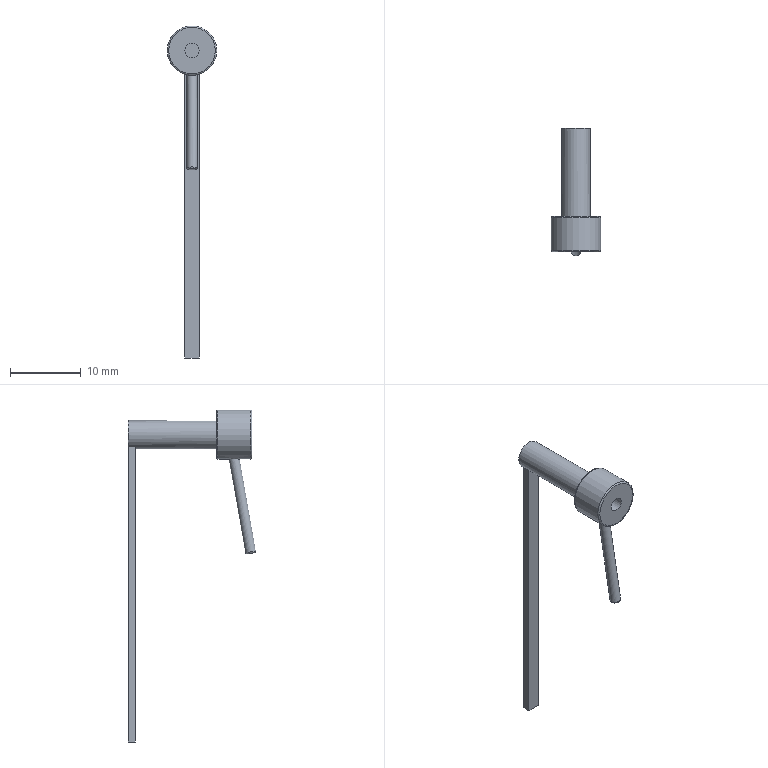Part | STEP file | 1-35.1 | 1 solid | 16 faces | box 7 x 18.051 x 47 mm | volume 449.87 mm3 | plane 9 | cylinder 4 | torus 3 | commonest cylinder face diameters 1.5 x1 2 x1 4 x1 7 x1
STEP:
#1=CARTESIAN_POINT('',(0.,0.,0.));
#2=DIRECTION('',(0.,0.,1.));
#3=DIRECTION('',(1.,0.,0.));
#4=AXIS2_PLACEMENT_3D('',#1,#2,#3);
#5=CARTESIAN_POINT('',(-1.,11.5,-1.732));
#6=VERTEX_POINT('',#5);
#7=CARTESIAN_POINT('',(1.,11.5,-1.732));
#8=VERTEX_POINT('',#7);
#9=CARTESIAN_POINT('',(0.,11.5,0.));
#10=DIRECTION('',(0.,-1.,0.));
#11=DIRECTION('',(-0.5,0.,-0.866));
#12=AXIS2_PLACEMENT_3D('',#9,#10,#11);
#13=CIRCLE('',#12,2.);
#14=CARTESIAN_POINT('',(0.,0.,0.));
#15=DIRECTION('',(0.,1.,0.));
#16=DIRECTION('',(1.,0.,0.));
#17=AXIS2_PLACEMENT_3D('',#14,#15,#16);
#18=CYLINDRICAL_SURFACE('',#17,2.);
#19=CARTESIAN_POINT('',(2.094,11.5));
#20=DIRECTION('',(-1.,0.));
#21=VECTOR('',#20,1.);
#22=LINE('',#19,#21);
#23=(GEOMETRIC_REPRESENTATION_CONTEXT(2)PARAMETRIC_REPRESENTATION_CONTEXT()REPRESENTATION_CONTEXT('',''));
#24=DEFINITIONAL_REPRESENTATION('',(#22),#23);
#25=PCURVE('',#18,#24);
#26=CARTESIAN_POINT('',(-20.242,11.5,-20.194));
#27=DIRECTION('',(0.,1.,0.));
#28=DIRECTION('',(-1.,0.,0.));
#29=AXIS2_PLACEMENT_3D('',#26,#27,#28);
#30=PLANE('',#29);
#31=CARTESIAN_POINT('',(-19.242,18.462));
#32=CARTESIAN_POINT('',(-22.242,16.73));
#33=CARTESIAN_POINT('',(-22.242,20.194));
#34=CARTESIAN_POINT('',(-22.242,23.658));
#35=CARTESIAN_POINT('',(-19.242,21.926));
#36=CARTESIAN_POINT('',(-16.242,20.194));
#37=CARTESIAN_POINT('',(-19.242,18.462));
#38=(BOUNDED_CURVE()B_SPLINE_CURVE(2,(#31,#32,#33,#34,#35,#36,#37),.UNSPECIFIED.,.T.,.F.)B_SPLINE_CURVE_WITH_KNOTS((1,2,2,2,2,1),(-2.094,0.,2.094,4.189,6.283,8.378),.UNSPECIFIED.)CURVE()GEOMETRIC_REPRESENTATION_ITEM()RATIONAL_B_SPLINE_CURVE((1.,0.5,1.,0.5,1.,0.5,1.))REPRESENTATION_ITEM(''));
#39=(GEOMETRIC_REPRESENTATION_CONTEXT(2)PARAMETRIC_REPRESENTATION_CONTEXT()REPRESENTATION_CONTEXT('',''));
#40=DEFINITIONAL_REPRESENTATION('',(#38),#39);
#41=PCURVE('',#30,#40);
#42=SURFACE_CURVE('',#13,(#25,#41),.PCURVE_S1.);
#43=EDGE_CURVE('',#6,#8,#42,.T.);
#44=ORIENTED_EDGE('',*,*,#43,.T.);
#45=CARTESIAN_POINT('',(1.,12.5,-1.732));
#46=VERTEX_POINT('',#45);
#47=CARTESIAN_POINT('',(1.,11.5,-1.732));
#48=DIRECTION('',(0.,1.,0.));
#49=VECTOR('',#48,1.);
#50=LINE('',#47,#49);
#51=CARTESIAN_POINT('',(1.047,11.5));
#52=DIRECTION('',(0.,1.));
#53=VECTOR('',#52,1.);
#54=LINE('',#51,#53);
#55=(GEOMETRIC_REPRESENTATION_CONTEXT(2)PARAMETRIC_REPRESENTATION_CONTEXT()REPRESENTATION_CONTEXT('',''));
#56=DEFINITIONAL_REPRESENTATION('',(#54),#55);
#57=PCURVE('',#18,#56);
#58=CARTESIAN_POINT('',(1.,12.,-22.616));
#59=DIRECTION('',(1.,0.,0.));
#60=DIRECTION('',(0.,0.,-1.));
#61=AXIS2_PLACEMENT_3D('',#58,#59,#60);
#62=PLANE('',#61);
#63=CARTESIAN_POINT('',(-20.884,-0.5));
#64=DIRECTION('',(0.,1.));
#65=VECTOR('',#64,1.);
#66=LINE('',#63,#65);
#67=(GEOMETRIC_REPRESENTATION_CONTEXT(2)PARAMETRIC_REPRESENTATION_CONTEXT()REPRESENTATION_CONTEXT('',''));
#68=DEFINITIONAL_REPRESENTATION('',(#66),#67);
#69=PCURVE('',#62,#68);
#70=SURFACE_CURVE('',#50,(#57,#69),.PCURVE_S1.);
#71=EDGE_CURVE('',#8,#46,#70,.T.);
#72=ORIENTED_EDGE('',*,*,#71,.T.);
#73=CARTESIAN_POINT('',(2.,12.5,0.));
#74=VERTEX_POINT('',#73);
#75=CARTESIAN_POINT('',(0.,12.5,0.));
#76=DIRECTION('',(0.,1.,0.));
#77=DIRECTION('',(1.,0.,0.));
#78=AXIS2_PLACEMENT_3D('',#75,#76,#77);
#79=CIRCLE('',#78,2.);
#80=CARTESIAN_POINT('',(0.,12.5));
#81=DIRECTION('',(1.,0.));
#82=VECTOR('',#81,1.);
#83=LINE('',#80,#82);
#84=(GEOMETRIC_REPRESENTATION_CONTEXT(2)PARAMETRIC_REPRESENTATION_CONTEXT()REPRESENTATION_CONTEXT('',''));
#85=DEFINITIONAL_REPRESENTATION('',(#83),#84);
#86=PCURVE('',#18,#85);
#87=CARTESIAN_POINT('',(-20.242,12.5,-20.194));
#88=DIRECTION('',(0.,1.,0.));
#89=DIRECTION('',(-1.,0.,0.));
#90=AXIS2_PLACEMENT_3D('',#87,#88,#89);
#91=PLANE('',#90);
#92=CARTESIAN_POINT('',(-20.242,20.194));
#93=DIRECTION('',(-1.,0.));
#94=AXIS2_PLACEMENT_2D('',#92,#93);
#95=CIRCLE('',#94,2.);
#96=(GEOMETRIC_REPRESENTATION_CONTEXT(2)PARAMETRIC_REPRESENTATION_CONTEXT()REPRESENTATION_CONTEXT('',''));
#97=DEFINITIONAL_REPRESENTATION('',(#95),#96);
#98=PCURVE('',#91,#97);
#99=SURFACE_CURVE('',#79,(#86,#98),.PCURVE_S1.);
#100=EDGE_CURVE('',#74,#46,#99,.T.);
#101=ORIENTED_EDGE('',*,*,#100,.F.);
#102=CARTESIAN_POINT('',(2.,0.,0.));
#103=VERTEX_POINT('',#102);
#104=CARTESIAN_POINT('',(2.,0.,0.));
#105=DIRECTION('',(0.,1.,0.));
#106=VECTOR('',#105,1.);
#107=LINE('',#104,#106);
#108=CARTESIAN_POINT('',(0.,0.));
#109=DIRECTION('',(0.,1.));
#110=VECTOR('',#109,1.);
#111=LINE('',#108,#110);
#112=(GEOMETRIC_REPRESENTATION_CONTEXT(2)PARAMETRIC_REPRESENTATION_CONTEXT()REPRESENTATION_CONTEXT('',''));
#113=DEFINITIONAL_REPRESENTATION('',(#111),#112);
#114=PCURVE('',#18,#113);
#115=CARTESIAN_POINT('',(6.283,0.));
#116=DIRECTION('',(0.,1.));
#117=VECTOR('',#116,1.);
#118=LINE('',#115,#117);
#119=(GEOMETRIC_REPRESENTATION_CONTEXT(2)PARAMETRIC_REPRESENTATION_CONTEXT()REPRESENTATION_CONTEXT('',''));
#120=DEFINITIONAL_REPRESENTATION('',(#118),#119);
#121=PCURVE('',#18,#120);
#122=SEAM_CURVE('',#107,(#114,#121),.PCURVE_S1.);
#123=EDGE_CURVE('',#103,#74,#122,.T.);
#124=ORIENTED_EDGE('',*,*,#123,.F.);
#125=CARTESIAN_POINT('',(0.,0.,0.));
#126=DIRECTION('',(0.,-1.,0.));
#127=DIRECTION('',(1.,0.,0.));
#128=AXIS2_PLACEMENT_3D('',#125,#126,#127);
#129=CIRCLE('',#128,2.);
#130=CARTESIAN_POINT('',(6.283,0.));
#131=DIRECTION('',(-1.,0.));
#132=VECTOR('',#131,1.);
#133=LINE('',#130,#132);
#134=(GEOMETRIC_REPRESENTATION_CONTEXT(2)PARAMETRIC_REPRESENTATION_CONTEXT()REPRESENTATION_CONTEXT('',''));
#135=DEFINITIONAL_REPRESENTATION('',(#133),#134);
#136=PCURVE('',#18,#135);
#137=CARTESIAN_POINT('',(-0.9378,0.,0.));
#138=DIRECTION('',(0.,-1.,0.));
#139=DIRECTION('',(1.,0.,0.));
#140=AXIS2_PLACEMENT_3D('',#137,#138,#139);
#141=PLANE('',#140);
#142=CARTESIAN_POINT('',(0.9378,0.));
#143=DIRECTION('',(1.,0.));
#144=AXIS2_PLACEMENT_2D('',#142,#143);
#145=CIRCLE('',#144,2.);
#146=(GEOMETRIC_REPRESENTATION_CONTEXT(2)PARAMETRIC_REPRESENTATION_CONTEXT()REPRESENTATION_CONTEXT('',''));
#147=DEFINITIONAL_REPRESENTATION('',(#145),#146);
#148=PCURVE('',#141,#147);
#149=SURFACE_CURVE('',#129,(#136,#148),.PCURVE_S1.);
#150=EDGE_CURVE('',#103,#103,#149,.T.);
#151=ORIENTED_EDGE('',*,*,#150,.F.);
#152=ORIENTED_EDGE('',*,*,#123,.T.);
#153=CARTESIAN_POINT('',(-1.,12.5,-1.732));
#154=VERTEX_POINT('',#153);
#155=CARTESIAN_POINT('',(0.,12.5,0.));
#156=DIRECTION('',(0.,1.,0.));
#157=DIRECTION('',(-0.5,0.,-0.866));
#158=AXIS2_PLACEMENT_3D('',#155,#156,#157);
#159=CIRCLE('',#158,2.);
#160=CARTESIAN_POINT('',(2.094,12.5));
#161=DIRECTION('',(1.,0.));
#162=VECTOR('',#161,1.);
#163=LINE('',#160,#162);
#164=(GEOMETRIC_REPRESENTATION_CONTEXT(2)PARAMETRIC_REPRESENTATION_CONTEXT()REPRESENTATION_CONTEXT('',''));
#165=DEFINITIONAL_REPRESENTATION('',(#163),#164);
#166=PCURVE('',#18,#165);
#167=CARTESIAN_POINT('',(-20.242,20.194));
#168=DIRECTION('',(0.5,-0.866));
#169=AXIS2_PLACEMENT_2D('',#167,#168);
#170=CIRCLE('',#169,2.);
#171=(GEOMETRIC_REPRESENTATION_CONTEXT(2)PARAMETRIC_REPRESENTATION_CONTEXT()REPRESENTATION_CONTEXT('',''));
#172=DEFINITIONAL_REPRESENTATION('',(#170),#171);
#173=PCURVE('',#91,#172);
#174=SURFACE_CURVE('',#159,(#166,#173),.PCURVE_S1.);
#175=EDGE_CURVE('',#154,#74,#174,.T.);
#176=ORIENTED_EDGE('',*,*,#175,.F.);
#177=CARTESIAN_POINT('',(-1.,11.5,-1.732));
#178=DIRECTION('',(0.,1.,0.));
#179=VECTOR('',#178,1.);
#180=LINE('',#177,#179);
#181=CARTESIAN_POINT('',(2.094,11.5));
#182=DIRECTION('',(0.,1.));
#183=VECTOR('',#182,1.);
#184=LINE('',#181,#183);
#185=(GEOMETRIC_REPRESENTATION_CONTEXT(2)PARAMETRIC_REPRESENTATION_CONTEXT()REPRESENTATION_CONTEXT('',''));
#186=DEFINITIONAL_REPRESENTATION('',(#184),#185);
#187=PCURVE('',#18,#186);
#188=CARTESIAN_POINT('',(-1.,12.,-22.616));
#189=DIRECTION('',(-1.,0.,0.));
#190=DIRECTION('',(0.,0.,1.));
#191=AXIS2_PLACEMENT_3D('',#188,#189,#190);
#192=PLANE('',#191);
#193=CARTESIAN_POINT('',(20.884,-0.5));
#194=DIRECTION('',(0.,1.));
#195=VECTOR('',#194,1.);
#196=LINE('',#193,#195);
#197=(GEOMETRIC_REPRESENTATION_CONTEXT(2)PARAMETRIC_REPRESENTATION_CONTEXT()REPRESENTATION_CONTEXT('',''));
#198=DEFINITIONAL_REPRESENTATION('',(#196),#197);
#199=PCURVE('',#192,#198);
#200=SURFACE_CURVE('',#180,(#187,#199),.PCURVE_S1.);
#201=EDGE_CURVE('',#6,#154,#200,.T.);
#202=ORIENTED_EDGE('',*,*,#201,.F.);
#203=EDGE_LOOP('',(#44,#72,#101,#124,#151,#152,#176,#202));
#204=FACE_BOUND('',#203,.T.);
#205=ADVANCED_FACE('',(#204),#18,.T.);
#206=CARTESIAN_POINT('',(3.3,0.,0.));
#207=VERTEX_POINT('',#206);
#208=CARTESIAN_POINT('',(0.,0.,0.));
#209=DIRECTION('',(0.,1.,0.));
#210=DIRECTION('',(1.,0.,0.));
#211=AXIS2_PLACEMENT_3D('',#208,#209,#210);
#212=CIRCLE('',#211,3.3);
#213=CARTESIAN_POINT('',(4.238,0.));
#214=CARTESIAN_POINT('',(4.238,-5.716));
#215=CARTESIAN_POINT('',(-0.7122,-2.858));
#216=CARTESIAN_POINT('',(-5.662,0.));
#217=CARTESIAN_POINT('',(-0.7122,2.858));
#218=CARTESIAN_POINT('',(4.238,5.716));
#219=CARTESIAN_POINT('',(4.238,0.));
#220=(BOUNDED_CURVE()B_SPLINE_CURVE(2,(#213,#214,#215,#216,#217,#218,#219),.UNSPECIFIED.,.T.,.F.)B_SPLINE_CURVE_WITH_KNOTS((1,2,2,2,2,1),(-2.094,0.,2.094,4.189,6.283,8.378),.UNSPECIFIED.)CURVE()GEOMETRIC_REPRESENTATION_ITEM()RATIONAL_B_SPLINE_CURVE((1.,0.5,1.,0.5,1.,0.5,1.))REPRESENTATION_ITEM(''));
#221=(GEOMETRIC_REPRESENTATION_CONTEXT(2)PARAMETRIC_REPRESENTATION_CONTEXT()REPRESENTATION_CONTEXT('',''));
#222=DEFINITIONAL_REPRESENTATION('',(#220),#221);
#223=PCURVE('',#141,#222);
#224=CARTESIAN_POINT('',(0.,-0.2,0.));
#225=DIRECTION('',(0.,-1.,0.));
#226=DIRECTION('',(1.,0.,0.));
#227=AXIS2_PLACEMENT_3D('',#224,#225,#226);
#228=TOROIDAL_SURFACE('',#227,3.3,0.2);
#229=CARTESIAN_POINT('',(6.283,4.712));
#230=DIRECTION('',(-1.,0.));
#231=VECTOR('',#230,1.);
#232=LINE('',#229,#231);
#233=(GEOMETRIC_REPRESENTATION_CONTEXT(2)PARAMETRIC_REPRESENTATION_CONTEXT()REPRESENTATION_CONTEXT('',''));
#234=DEFINITIONAL_REPRESENTATION('',(#232),#233);
#235=PCURVE('',#228,#234);
#236=SURFACE_CURVE('',#212,(#223,#235),.PCURVE_S1.);
#237=EDGE_CURVE('',#207,#207,#236,.T.);
#238=ORIENTED_EDGE('',*,*,#237,.F.);
#239=EDGE_LOOP('',(#238));
#240=FACE_BOUND('',#239,.F.);
#241=ORIENTED_EDGE('',*,*,#150,.F.);
#242=EDGE_LOOP('',(#241));
#243=FACE_BOUND('',#242,.F.);
#244=ADVANCED_FACE('',(#240,#243),#141,.F.);
#245=ORIENTED_EDGE('',*,*,#237,.F.);
#246=CARTESIAN_POINT('',(3.5,-0.2,0.));
#247=VERTEX_POINT('',#246);
#248=CARTESIAN_POINT('',(3.3,-0.2,0.));
#249=DIRECTION('',(0.,0.,-1.));
#250=DIRECTION('',(0.,1.,0.));
#251=AXIS2_PLACEMENT_3D('',#248,#249,#250);
#252=CIRCLE('',#251,0.2);
#253=CARTESIAN_POINT('',(6.283,4.712));
#254=DIRECTION('',(0.,1.));
#255=VECTOR('',#254,1.);
#256=LINE('',#253,#255);
#257=(GEOMETRIC_REPRESENTATION_CONTEXT(2)PARAMETRIC_REPRESENTATION_CONTEXT()REPRESENTATION_CONTEXT('',''));
#258=DEFINITIONAL_REPRESENTATION('',(#256),#257);
#259=PCURVE('',#228,#258);
#260=CARTESIAN_POINT('',(0.,4.712));
#261=DIRECTION('',(0.,1.));
#262=VECTOR('',#261,1.);
#263=LINE('',#260,#262);
#264=(GEOMETRIC_REPRESENTATION_CONTEXT(2)PARAMETRIC_REPRESENTATION_CONTEXT()REPRESENTATION_CONTEXT('',''));
#265=DEFINITIONAL_REPRESENTATION('',(#263),#264);
#266=PCURVE('',#228,#265);
#267=SEAM_CURVE('',#252,(#259,#266),.PCURVE_S1.);
#268=EDGE_CURVE('',#207,#247,#267,.T.);
#269=ORIENTED_EDGE('',*,*,#268,.T.);
#270=CARTESIAN_POINT('',(0.,-0.2,0.));
#271=DIRECTION('',(0.,1.,0.));
#272=DIRECTION('',(1.,0.,0.));
#273=AXIS2_PLACEMENT_3D('',#270,#271,#272);
#274=CIRCLE('',#273,3.5);
#275=CARTESIAN_POINT('',(6.283,6.283));
#276=DIRECTION('',(-1.,0.));
#277=VECTOR('',#276,1.);
#278=LINE('',#275,#277);
#279=(GEOMETRIC_REPRESENTATION_CONTEXT(2)PARAMETRIC_REPRESENTATION_CONTEXT()REPRESENTATION_CONTEXT('',''));
#280=DEFINITIONAL_REPRESENTATION('',(#278),#279);
#281=PCURVE('',#228,#280);
#282=CARTESIAN_POINT('',(0.,0.,0.));
#283=DIRECTION('',(0.,-1.,0.));
#284=DIRECTION('',(1.,0.,0.));
#285=AXIS2_PLACEMENT_3D('',#282,#283,#284);
#286=CYLINDRICAL_SURFACE('',#285,3.5);
#287=CARTESIAN_POINT('',(6.283,0.2));
#288=DIRECTION('',(-1.,0.));
#289=VECTOR('',#288,1.);
#290=LINE('',#287,#289);
#291=(GEOMETRIC_REPRESENTATION_CONTEXT(2)PARAMETRIC_REPRESENTATION_CONTEXT()REPRESENTATION_CONTEXT('',''));
#292=DEFINITIONAL_REPRESENTATION('',(#290),#291);
#293=PCURVE('',#286,#292);
#294=SURFACE_CURVE('',#274,(#281,#293),.PCURVE_S1.);
#295=EDGE_CURVE('',#247,#247,#294,.T.);
#296=ORIENTED_EDGE('',*,*,#295,.T.);
#297=ORIENTED_EDGE('',*,*,#268,.F.);
#298=EDGE_LOOP('',(#245,#269,#296,#297));
#299=FACE_BOUND('',#298,.T.);
#300=ADVANCED_FACE('',(#299),#228,.T.);
#301=CARTESIAN_POINT('',(3.3,-5.,0.));
#302=VERTEX_POINT('',#301);
#303=CARTESIAN_POINT('',(3.5,-4.8,0.));
#304=VERTEX_POINT('',#303);
#305=CARTESIAN_POINT('',(3.3,-4.8,0.));
#306=DIRECTION('',(0.,0.,1.));
#307=DIRECTION('',(0.,-1.,0.));
#308=AXIS2_PLACEMENT_3D('',#305,#306,#307);
#309=CIRCLE('',#308,0.2);
#310=CARTESIAN_POINT('',(0.,-4.8,0.));
#311=DIRECTION('',(0.,-1.,0.));
#312=DIRECTION('',(1.,0.,0.));
#313=AXIS2_PLACEMENT_3D('',#310,#311,#312);
#314=TOROIDAL_SURFACE('',#313,3.3,0.2);
#315=CARTESIAN_POINT('',(0.,1.571));
#316=DIRECTION('',(0.,-1.));
#317=VECTOR('',#316,1.);
#318=LINE('',#315,#317);
#319=(GEOMETRIC_REPRESENTATION_CONTEXT(2)PARAMETRIC_REPRESENTATION_CONTEXT()REPRESENTATION_CONTEXT('',''));
#320=DEFINITIONAL_REPRESENTATION('',(#318),#319);
#321=PCURVE('',#314,#320);
#322=CARTESIAN_POINT('',(6.283,1.571));
#323=DIRECTION('',(0.,-1.));
#324=VECTOR('',#323,1.);
#325=LINE('',#322,#324);
#326=(GEOMETRIC_REPRESENTATION_CONTEXT(2)PARAMETRIC_REPRESENTATION_CONTEXT()REPRESENTATION_CONTEXT('',''));
#327=DEFINITIONAL_REPRESENTATION('',(#325),#326);
#328=PCURVE('',#314,#327);
#329=SEAM_CURVE('',#309,(#321,#328),.PCURVE_S1.);
#330=EDGE_CURVE('',#302,#304,#329,.T.);
#331=ORIENTED_EDGE('',*,*,#330,.T.);
#332=CARTESIAN_POINT('',(0.,-4.8,0.));
#333=DIRECTION('',(0.,1.,0.));
#334=DIRECTION('',(1.,0.,0.));
#335=AXIS2_PLACEMENT_3D('',#332,#333,#334);
#336=CIRCLE('',#335,3.5);
#337=CARTESIAN_POINT('',(6.283,0.));
#338=DIRECTION('',(-1.,0.));
#339=VECTOR('',#338,1.);
#340=LINE('',#337,#339);
#341=(GEOMETRIC_REPRESENTATION_CONTEXT(2)PARAMETRIC_REPRESENTATION_CONTEXT()REPRESENTATION_CONTEXT('',''));
#342=DEFINITIONAL_REPRESENTATION('',(#340),#341);
#343=PCURVE('',#314,#342);
#344=CARTESIAN_POINT('',(6.283,4.8));
#345=DIRECTION('',(-1.,0.));
#346=VECTOR('',#345,1.);
#347=LINE('',#344,#346);
#348=(GEOMETRIC_REPRESENTATION_CONTEXT(2)PARAMETRIC_REPRESENTATION_CONTEXT()REPRESENTATION_CONTEXT('',''));
#349=DEFINITIONAL_REPRESENTATION('',(#347),#348);
#350=PCURVE('',#286,#349);
#351=SURFACE_CURVE('',#336,(#343,#350),.PCURVE_S1.);
#352=EDGE_CURVE('',#304,#304,#351,.T.);
#353=ORIENTED_EDGE('',*,*,#352,.F.);
#354=ORIENTED_EDGE('',*,*,#330,.F.);
#355=CARTESIAN_POINT('',(0.,-5.,0.));
#356=DIRECTION('',(0.,1.,0.));
#357=DIRECTION('',(1.,0.,0.));
#358=AXIS2_PLACEMENT_3D('',#355,#356,#357);
#359=CIRCLE('',#358,3.3);
#360=CARTESIAN_POINT('',(6.283,1.571));
#361=DIRECTION('',(-1.,0.));
#362=VECTOR('',#361,1.);
#363=LINE('',#360,#362);
#364=(GEOMETRIC_REPRESENTATION_CONTEXT(2)PARAMETRIC_REPRESENTATION_CONTEXT()REPRESENTATION_CONTEXT('',''));
#365=DEFINITIONAL_REPRESENTATION('',(#363),#364);
#366=PCURVE('',#314,#365);
#367=CARTESIAN_POINT('',(-0.9378,-5.,0.));
#368=DIRECTION('',(0.,-1.,0.));
#369=DIRECTION('',(1.,0.,0.));
#370=AXIS2_PLACEMENT_3D('',#367,#368,#369);
#371=PLANE('',#370);
#372=CARTESIAN_POINT('',(4.238,0.));
#373=CARTESIAN_POINT('',(4.238,-5.716));
#374=CARTESIAN_POINT('',(-0.7122,-2.858));
#375=CARTESIAN_POINT('',(-5.662,0.));
#376=CARTESIAN_POINT('',(-0.7122,2.858));
#377=CARTESIAN_POINT('',(4.238,5.716));
#378=CARTESIAN_POINT('',(4.238,0.));
#379=(BOUNDED_CURVE()B_SPLINE_CURVE(2,(#372,#373,#374,#375,#376,#377,#378),.UNSPECIFIED.,.T.,.F.)B_SPLINE_CURVE_WITH_KNOTS((1,2,2,2,2,1),(-2.094,0.,2.094,4.189,6.283,8.378),.UNSPECIFIED.)CURVE()GEOMETRIC_REPRESENTATION_ITEM()RATIONAL_B_SPLINE_CURVE((1.,0.5,1.,0.5,1.,0.5,1.))REPRESENTATION_ITEM(''));
#380=(GEOMETRIC_REPRESENTATION_CONTEXT(2)PARAMETRIC_REPRESENTATION_CONTEXT()REPRESENTATION_CONTEXT('',''));
#381=DEFINITIONAL_REPRESENTATION('',(#379),#380);
#382=PCURVE('',#371,#381);
#383=SURFACE_CURVE('',#359,(#366,#382),.PCURVE_S1.);
#384=EDGE_CURVE('',#302,#302,#383,.T.);
#385=ORIENTED_EDGE('',*,*,#384,.T.);
#386=EDGE_LOOP('',(#331,#353,#354,#385));
#387=FACE_BOUND('',#386,.T.);
#388=ADVANCED_FACE('',(#387),#314,.T.);
#389=ORIENTED_EDGE('',*,*,#384,.F.);
#390=EDGE_LOOP('',(#389));
#391=FACE_BOUND('',#390,.T.);
#392=CARTESIAN_POINT('',(1.,-5.,0.));
#393=VERTEX_POINT('',#392);
#394=CARTESIAN_POINT('',(0.,-5.,0.));
#395=DIRECTION('',(0.,-1.,0.));
#396=DIRECTION('',(1.,0.,0.));
#397=AXIS2_PLACEMENT_3D('',#394,#395,#396);
#398=CIRCLE('',#397,1.);
#399=CARTESIAN_POINT('',(0.9378,0.));
#400=DIRECTION('',(1.,0.));
#401=AXIS2_PLACEMENT_2D('',#399,#400);
#402=CIRCLE('',#401,1.);
#403=(GEOMETRIC_REPRESENTATION_CONTEXT(2)PARAMETRIC_REPRESENTATION_CONTEXT()REPRESENTATION_CONTEXT('',''));
#404=DEFINITIONAL_REPRESENTATION('',(#402),#403);
#405=PCURVE('',#371,#404);
#406=CARTESIAN_POINT('',(0.,-5.,0.));
#407=DIRECTION('',(0.,1.,0.));
#408=DIRECTION('',(1.,0.,0.));
#409=AXIS2_PLACEMENT_3D('',#406,#407,#408);
#410=CYLINDRICAL_SURFACE('',#409,1.);
#411=CARTESIAN_POINT('',(6.283,0.));
#412=DIRECTION('',(-1.,0.));
#413=VECTOR('',#412,1.);
#414=LINE('',#411,#413);
#415=(GEOMETRIC_REPRESENTATION_CONTEXT(2)PARAMETRIC_REPRESENTATION_CONTEXT()REPRESENTATION_CONTEXT('',''));
#416=DEFINITIONAL_REPRESENTATION('',(#414),#415);
#417=PCURVE('',#410,#416);
#418=SURFACE_CURVE('',#398,(#405,#417),.PCURVE_S1.);
#419=EDGE_CURVE('',#393,#393,#418,.T.);
#420=ORIENTED_EDGE('',*,*,#419,.F.);
#421=EDGE_LOOP('',(#420));
#422=FACE_BOUND('',#421,.T.);
#423=ADVANCED_FACE('',(#391,#422),#371,.T.);
#424=CARTESIAN_POINT('',(1.,-3.,0.));
#425=VERTEX_POINT('',#424);
#426=CARTESIAN_POINT('',(1.,-5.,0.));
#427=DIRECTION('',(0.,1.,0.));
#428=VECTOR('',#427,1.);
#429=LINE('',#426,#428);
#430=CARTESIAN_POINT('',(6.283,0.));
#431=DIRECTION('',(0.,1.));
#432=VECTOR('',#431,1.);
#433=LINE('',#430,#432);
#434=(GEOMETRIC_REPRESENTATION_CONTEXT(2)PARAMETRIC_REPRESENTATION_CONTEXT()REPRESENTATION_CONTEXT('',''));
#435=DEFINITIONAL_REPRESENTATION('',(#433),#434);
#436=PCURVE('',#410,#435);
#437=CARTESIAN_POINT('',(0.,0.));
#438=DIRECTION('',(0.,1.));
#439=VECTOR('',#438,1.);
#440=LINE('',#437,#439);
#441=(GEOMETRIC_REPRESENTATION_CONTEXT(2)PARAMETRIC_REPRESENTATION_CONTEXT()REPRESENTATION_CONTEXT('',''));
#442=DEFINITIONAL_REPRESENTATION('',(#440),#441);
#443=PCURVE('',#410,#442);
#444=SEAM_CURVE('',#429,(#436,#443),.PCURVE_S1.);
#445=EDGE_CURVE('',#393,#425,#444,.T.);
#446=ORIENTED_EDGE('',*,*,#445,.T.);
#447=CARTESIAN_POINT('',(0.,-3.,0.));
#448=DIRECTION('',(0.,-1.,0.));
#449=DIRECTION('',(1.,0.,0.));
#450=AXIS2_PLACEMENT_3D('',#447,#448,#449);
#451=CIRCLE('',#450,1.);
#452=CARTESIAN_POINT('',(6.283,2.));
#453=DIRECTION('',(-1.,0.));
#454=VECTOR('',#453,1.);
#455=LINE('',#452,#454);
#456=(GEOMETRIC_REPRESENTATION_CONTEXT(2)PARAMETRIC_REPRESENTATION_CONTEXT()REPRESENTATION_CONTEXT('',''));
#457=DEFINITIONAL_REPRESENTATION('',(#455),#456);
#458=PCURVE('',#410,#457);
#459=CARTESIAN_POINT('',(-0.2679,-3.,0.));
#460=DIRECTION('',(0.,-1.,0.));
#461=DIRECTION('',(1.,0.,0.));
#462=AXIS2_PLACEMENT_3D('',#459,#460,#461);
#463=PLANE('',#462);
#464=CARTESIAN_POINT('',(0.2679,0.));
#465=DIRECTION('',(1.,0.));
#466=AXIS2_PLACEMENT_2D('',#464,#465);
#467=CIRCLE('',#466,1.);
#468=(GEOMETRIC_REPRESENTATION_CONTEXT(2)PARAMETRIC_REPRESENTATION_CONTEXT()REPRESENTATION_CONTEXT('',''));
#469=DEFINITIONAL_REPRESENTATION('',(#467),#468);
#470=PCURVE('',#463,#469);
#471=SURFACE_CURVE('',#451,(#458,#470),.PCURVE_S1.);
#472=EDGE_CURVE('',#425,#425,#471,.T.);
#473=ORIENTED_EDGE('',*,*,#472,.T.);
#474=ORIENTED_EDGE('',*,*,#445,.F.);
#475=ORIENTED_EDGE('',*,*,#419,.F.);
#476=EDGE_LOOP('',(#446,#473,#474,#475));
#477=FACE_BOUND('',#476,.F.);
#478=ADVANCED_FACE('',(#477),#410,.F.);
#479=ORIENTED_EDGE('',*,*,#472,.T.);
#480=EDGE_LOOP('',(#479));
#481=FACE_BOUND('',#480,.T.);
#482=ADVANCED_FACE('',(#481),#463,.T.);
#483=CARTESIAN_POINT('',(3.5,-0.2,0.));
#484=DIRECTION('',(0.,-1.,0.));
#485=VECTOR('',#484,1.);
#486=LINE('',#483,#485);
#487=CARTESIAN_POINT('',(6.283,0.2));
#488=DIRECTION('',(0.,1.));
#489=VECTOR('',#488,1.);
#490=LINE('',#487,#489);
#491=(GEOMETRIC_REPRESENTATION_CONTEXT(2)PARAMETRIC_REPRESENTATION_CONTEXT()REPRESENTATION_CONTEXT('',''));
#492=DEFINITIONAL_REPRESENTATION('',(#490),#491);
#493=PCURVE('',#286,#492);
#494=CARTESIAN_POINT('',(0.,0.2));
#495=DIRECTION('',(0.,1.));
#496=VECTOR('',#495,1.);
#497=LINE('',#494,#496);
#498=(GEOMETRIC_REPRESENTATION_CONTEXT(2)PARAMETRIC_REPRESENTATION_CONTEXT()REPRESENTATION_CONTEXT('',''));
#499=DEFINITIONAL_REPRESENTATION('',(#497),#498);
#500=PCURVE('',#286,#499);
#501=SEAM_CURVE('',#486,(#493,#500),.PCURVE_S1.);
#502=EDGE_CURVE('',#247,#304,#501,.T.);
#503=ORIENTED_EDGE('',*,*,#502,.T.);
#504=ORIENTED_EDGE('',*,*,#352,.T.);
#505=ORIENTED_EDGE('',*,*,#502,.F.);
#506=ORIENTED_EDGE('',*,*,#295,.F.);
#507=EDGE_LOOP('',(#503,#504,#505,#506));
#508=FACE_BOUND('',#507,.T.);
#509=CARTESIAN_POINT('',(-0.75,-2.486,-3.419));
#510=VERTEX_POINT('',#509);
#511=CARTESIAN_POINT('',(-0.75,-2.486,-3.419));
#512=CARTESIAN_POINT('',(-0.75,-2.376,-3.419));
#513=CARTESIAN_POINT('',(-0.6794,-2.045,-3.434));
#514=CARTESIAN_POINT('',(-0.4093,-1.822,-3.482));
#515=CARTESIAN_POINT('',(0.1996,-1.656,-3.517));
#516=CARTESIAN_POINT('',(0.6137,-1.883,-3.448));
#517=CARTESIAN_POINT('',(0.8541,-2.766,-3.397));
#518=CARTESIAN_POINT('',(0.4949,-3.262,-3.5));
#519=CARTESIAN_POINT('',(-0.2674,-3.262,-3.5));
#520=CARTESIAN_POINT('',(-0.6454,-3.022,-3.442));
#521=CARTESIAN_POINT('',(-0.75,-2.62,-3.419));
#522=CARTESIAN_POINT('',(-0.75,-2.486,-3.419));
#523=B_SPLINE_CURVE_WITH_KNOTS('',3,(#511,#512,#513,#514,#515,#516,#517,#518,#519,#520,#521,#522),.UNSPECIFIED.,.T.,.F.,(1,3,1,2,2,2,1,3,1),(-0.3333,0.,0.2702,0.8105,1.846,3.08,3.747,4.08,4.35),.UNSPECIFIED.);
#524=CARTESIAN_POINT('',(4.496,2.486));
#525=CARTESIAN_POINT('',(4.496,2.448));
#526=CARTESIAN_POINT('',(4.498,2.372));
#527=CARTESIAN_POINT('',(4.505,2.262));
#528=CARTESIAN_POINT('',(4.517,2.157));
#529=CARTESIAN_POINT('',(4.533,2.061));
#530=CARTESIAN_POINT('',(4.554,1.975));
#531=CARTESIAN_POINT('',(4.577,1.9));
#532=CARTESIAN_POINT('',(4.604,1.837));
#533=CARTESIAN_POINT('',(4.632,1.789));
#534=CARTESIAN_POINT('',(4.663,1.755));
#535=CARTESIAN_POINT('',(4.694,1.738));
#536=CARTESIAN_POINT('',(4.724,1.737));
#537=CARTESIAN_POINT('',(4.754,1.749));
#538=CARTESIAN_POINT('',(4.783,1.776));
#539=CARTESIAN_POINT('',(4.81,1.816));
#540=CARTESIAN_POINT('',(4.836,1.868));
#541=CARTESIAN_POINT('',(4.859,1.932));
#542=CARTESIAN_POINT('',(4.88,2.008));
#543=CARTESIAN_POINT('',(4.897,2.094));
#544=CARTESIAN_POINT('',(4.912,2.189));
#545=CARTESIAN_POINT('',(4.922,2.295));
#546=CARTESIAN_POINT('',(4.928,2.404));
#547=CARTESIAN_POINT('',(4.929,2.511));
#548=CARTESIAN_POINT('',(4.926,2.617));
#549=CARTESIAN_POINT('',(4.919,2.719));
#550=CARTESIAN_POINT('',(4.908,2.816));
#551=CARTESIAN_POINT('',(4.893,2.907));
#552=CARTESIAN_POINT('',(4.876,2.991));
#553=CARTESIAN_POINT('',(4.856,3.065));
#554=CARTESIAN_POINT('',(4.833,3.13));
#555=CARTESIAN_POINT('',(4.807,3.184));
#556=CARTESIAN_POINT('',(4.78,3.225));
#557=CARTESIAN_POINT('',(4.75,3.252));
#558=CARTESIAN_POINT('',(4.719,3.264));
#559=CARTESIAN_POINT('',(4.687,3.259));
#560=CARTESIAN_POINT('',(4.657,3.236));
#561=CARTESIAN_POINT('',(4.627,3.197));
#562=CARTESIAN_POINT('',(4.599,3.144));
#563=CARTESIAN_POINT('',(4.574,3.077));
#564=CARTESIAN_POINT('',(4.551,2.999));
#565=CARTESIAN_POINT('',(4.532,2.91));
#566=CARTESIAN_POINT('',(4.516,2.812));
#567=CARTESIAN_POINT('',(4.505,2.707));
#568=CARTESIAN_POINT('',(4.498,2.598));
#569=CARTESIAN_POINT('',(4.496,2.523));
#570=CARTESIAN_POINT('',(4.496,2.486));
#571=B_SPLINE_CURVE_WITH_KNOTS('',3,(#524,#525,#526,#527,#528,#529,#530,#531,#532,#533,#534,#535,#536,#537,#538,#539,#540,#541,#542,#543,#544,#545,#546,#547,#548,#549,#550,#551,#552,#553,#554,#555,#556,#557,#558,#559,#560,#561,#562,#563,#564,#565,#566,#567,#568,#569,#570),.UNSPECIFIED.,.T.,.F.,(4,1,1,1,1,1,1,1,1,1,1,1,1,1,1,1,1,1,1,1,1,1,1,1,1,1,1,1,1,1,1,1,1,1,1,1,1,1,1,1,1,1,1,1,4),(0.,0.09273,0.1855,0.2782,0.3709,0.4636,0.5564,0.6491,0.7418,0.8345,0.9273,1.02,1.113,1.205,1.298,1.391,1.484,1.576,1.669,1.762,1.855,1.947,2.04,2.133,2.225,2.318,2.411,2.504,2.596,2.689,2.782,2.875,2.967,3.06,3.153,3.245,3.338,3.431,3.524,3.616,3.709,3.802,3.895,3.987,4.08),.QUASI_UNIFORM_KNOTS.);
#572=(GEOMETRIC_REPRESENTATION_CONTEXT(2)PARAMETRIC_REPRESENTATION_CONTEXT()REPRESENTATION_CONTEXT('',''));
#573=DEFINITIONAL_REPRESENTATION('',(#571),#572);
#574=PCURVE('',#286,#573);
#575=CARTESIAN_POINT('',(0.,-0.6267,7.124));
#576=DIRECTION('',(0.,-0.1736,-0.9848));
#577=DIRECTION('',(-1.,0.,0.));
#578=AXIS2_PLACEMENT_3D('',#575,#576,#577);
#579=CYLINDRICAL_SURFACE('',#578,0.75);
#580=CARTESIAN_POINT('',(0.,10.705));
#581=CARTESIAN_POINT('',(0.04965,10.699));
#582=CARTESIAN_POINT('',(0.1492,10.687));
#583=CARTESIAN_POINT('',(0.2987,10.673));
#584=CARTESIAN_POINT('',(0.4476,10.662));
#585=CARTESIAN_POINT('',(0.5959,10.656));
#586=CARTESIAN_POINT('',(0.7444,10.653));
#587=CARTESIAN_POINT('',(0.8929,10.652));
#588=CARTESIAN_POINT('',(1.042,10.652));
#589=CARTESIAN_POINT('',(1.19,10.654));
#590=CARTESIAN_POINT('',(1.339,10.655));
#591=CARTESIAN_POINT('',(1.484,10.655));
#592=CARTESIAN_POINT('',(1.626,10.654));
#593=CARTESIAN_POINT('',(1.766,10.652));
#594=CARTESIAN_POINT('',(1.904,10.651));
#595=CARTESIAN_POINT('',(2.042,10.649));
#596=CARTESIAN_POINT('',(2.18,10.649));
#597=CARTESIAN_POINT('',(2.318,10.65));
#598=CARTESIAN_POINT('',(2.457,10.653));
#599=CARTESIAN_POINT('',(2.597,10.658));
#600=CARTESIAN_POINT('',(2.74,10.666));
#601=CARTESIAN_POINT('',(2.888,10.677));
#602=CARTESIAN_POINT('',(3.034,10.692));
#603=CARTESIAN_POINT('',(3.175,10.711));
#604=CARTESIAN_POINT('',(3.313,10.732));
#605=CARTESIAN_POINT('',(3.449,10.756));
#606=CARTESIAN_POINT('',(3.584,10.781));
#607=CARTESIAN_POINT('',(3.718,10.806));
#608=CARTESIAN_POINT('',(3.852,10.83));
#609=CARTESIAN_POINT('',(3.986,10.853));
#610=CARTESIAN_POINT('',(4.121,10.874));
#611=CARTESIAN_POINT('',(4.257,10.892));
#612=CARTESIAN_POINT('',(4.394,10.907));
#613=CARTESIAN_POINT('',(4.535,10.917));
#614=CARTESIAN_POINT('',(4.68,10.921));
#615=CARTESIAN_POINT('',(4.829,10.919));
#616=CARTESIAN_POINT('',(4.975,10.91));
#617=CARTESIAN_POINT('',(5.121,10.895));
#618=CARTESIAN_POINT('',(5.267,10.876));
#619=CARTESIAN_POINT('',(5.412,10.853));
#620=CARTESIAN_POINT('',(5.557,10.828));
#621=CARTESIAN_POINT('',(5.701,10.802));
#622=CARTESIAN_POINT('',(5.846,10.775));
#623=CARTESIAN_POINT('',(5.991,10.75));
#624=CARTESIAN_POINT('',(6.137,10.726));
#625=CARTESIAN_POINT('',(6.234,10.712));
#626=CARTESIAN_POINT('',(6.283,10.705));
#627=B_SPLINE_CURVE_WITH_KNOTS('',3,(#580,#581,#582,#583,#584,#585,#586,#587,#588,#589,#590,#591,#592,#593,#594,#595,#596,#597,#598,#599,#600,#601,#602,#603,#604,#605,#606,#607,#608,#609,#610,#611,#612,#613,#614,#615,#616,#617,#618,#619,#620,#621,#622,#623,#624,#625,#626),.UNSPECIFIED.,.F.,.F.,(4,1,1,1,1,1,1,1,1,1,1,1,1,1,1,1,1,1,1,1,1,1,1,1,1,1,1,1,1,1,1,1,1,1,1,1,1,1,1,1,1,1,1,1,4),(0.,0.09273,0.1855,0.2782,0.3709,0.4636,0.5564,0.6491,0.7418,0.8345,0.9273,1.02,1.113,1.205,1.298,1.391,1.484,1.576,1.669,1.762,1.855,1.947,2.04,2.133,2.225,2.318,2.411,2.504,2.596,2.689,2.782,2.875,2.967,3.06,3.153,3.245,3.338,3.431,3.524,3.616,3.709,3.802,3.895,3.987,4.08),.QUASI_UNIFORM_KNOTS.);
#628=(GEOMETRIC_REPRESENTATION_CONTEXT(2)PARAMETRIC_REPRESENTATION_CONTEXT()REPRESENTATION_CONTEXT('',''));
#629=DEFINITIONAL_REPRESENTATION('',(#627),#628);
#630=PCURVE('',#579,#629);
#631=SURFACE_CURVE('',#523,(#574,#630),.PCURVE_S1.);
#632=EDGE_CURVE('',#510,#510,#631,.T.);
#633=ORIENTED_EDGE('',*,*,#632,.F.);
#634=EDGE_LOOP('',(#633));
#635=FACE_BOUND('',#634,.T.);
#636=ADVANCED_FACE('',(#508,#635),#286,.T.);
#637=CARTESIAN_POINT('',(-0.75,-4.81,-16.598));
#638=VERTEX_POINT('',#637);
#639=CARTESIAN_POINT('',(-0.75,-4.81,-16.598));
#640=DIRECTION('',(0.,0.1736,0.9848));
#641=VECTOR('',#640,1.);
#642=LINE('',#639,#641);
#643=CARTESIAN_POINT('',(6.283,24.088));
#644=DIRECTION('',(0.,-1.));
#645=VECTOR('',#644,1.);
#646=LINE('',#643,#645);
#647=(GEOMETRIC_REPRESENTATION_CONTEXT(2)PARAMETRIC_REPRESENTATION_CONTEXT()REPRESENTATION_CONTEXT('',''));
#648=DEFINITIONAL_REPRESENTATION('',(#646),#647);
#649=PCURVE('',#579,#648);
#650=CARTESIAN_POINT('',(0.,24.088));
#651=DIRECTION('',(0.,-1.));
#652=VECTOR('',#651,1.);
#653=LINE('',#650,#652);
#654=(GEOMETRIC_REPRESENTATION_CONTEXT(2)PARAMETRIC_REPRESENTATION_CONTEXT()REPRESENTATION_CONTEXT('',''));
#655=DEFINITIONAL_REPRESENTATION('',(#653),#654);
#656=PCURVE('',#579,#655);
#657=SEAM_CURVE('',#642,(#649,#656),.PCURVE_S1.);
#658=EDGE_CURVE('',#638,#510,#657,.T.);
#659=ORIENTED_EDGE('',*,*,#658,.F.);
#660=CARTESIAN_POINT('',(0.,-4.81,-16.598));
#661=DIRECTION('',(0.,0.1736,0.9848));
#662=DIRECTION('',(-1.,0.,0.));
#663=AXIS2_PLACEMENT_3D('',#660,#661,#662);
#664=CIRCLE('',#663,0.75);
#665=CARTESIAN_POINT('',(6.283,24.088));
#666=DIRECTION('',(-1.,0.));
#667=VECTOR('',#666,1.);
#668=LINE('',#665,#667);
#669=(GEOMETRIC_REPRESENTATION_CONTEXT(2)PARAMETRIC_REPRESENTATION_CONTEXT()REPRESENTATION_CONTEXT('',''));
#670=DEFINITIONAL_REPRESENTATION('',(#668),#669);
#671=PCURVE('',#579,#670);
#672=CARTESIAN_POINT('',(0.,-4.81,-16.598));
#673=DIRECTION('',(0.,-0.1736,-0.9848));
#674=DIRECTION('',(-1.,0.,0.));
#675=AXIS2_PLACEMENT_3D('',#672,#673,#674);
#676=TOROIDAL_SURFACE('',#675,0.55,0.2);
#677=CARTESIAN_POINT('',(6.283,0.));
#678=DIRECTION('',(-1.,0.));
#679=VECTOR('',#678,1.);
#680=LINE('',#677,#679);
#681=(GEOMETRIC_REPRESENTATION_CONTEXT(2)PARAMETRIC_REPRESENTATION_CONTEXT()REPRESENTATION_CONTEXT('',''));
#682=DEFINITIONAL_REPRESENTATION('',(#680),#681);
#683=PCURVE('',#676,#682);
#684=SURFACE_CURVE('',#664,(#671,#683),.PCURVE_S1.);
#685=EDGE_CURVE('',#638,#638,#684,.T.);
#686=ORIENTED_EDGE('',*,*,#685,.T.);
#687=ORIENTED_EDGE('',*,*,#658,.T.);
#688=ORIENTED_EDGE('',*,*,#632,.T.);
#689=EDGE_LOOP('',(#659,#686,#687,#688));
#690=FACE_BOUND('',#689,.T.);
#691=ADVANCED_FACE('',(#690),#579,.T.);
#692=CARTESIAN_POINT('',(-0.55,-4.844,-16.795));
#693=VERTEX_POINT('',#692);
#694=CARTESIAN_POINT('',(0.,-4.844,-16.795));
#695=DIRECTION('',(0.,0.1736,0.9848));
#696=DIRECTION('',(-1.,0.,0.));
#697=AXIS2_PLACEMENT_3D('',#694,#695,#696);
#698=CIRCLE('',#697,0.55);
#699=CARTESIAN_POINT('',(0.,-4.844,-16.795));
#700=DIRECTION('',(0.,-0.1736,-0.9848));
#701=DIRECTION('',(1.,0.,0.));
#702=AXIS2_PLACEMENT_3D('',#699,#700,#701);
#703=PLANE('',#702);
#704=CARTESIAN_POINT('',(-0.55,0.));
#705=CARTESIAN_POINT('',(-0.55,0.9526));
#706=CARTESIAN_POINT('',(0.275,0.4763));
#707=CARTESIAN_POINT('',(1.1,0.));
#708=CARTESIAN_POINT('',(0.275,-0.4763));
#709=CARTESIAN_POINT('',(-0.55,-0.9526));
#710=CARTESIAN_POINT('',(-0.55,0.));
#711=(BOUNDED_CURVE()B_SPLINE_CURVE(2,(#704,#705,#706,#707,#708,#709,#710),.UNSPECIFIED.,.T.,.F.)B_SPLINE_CURVE_WITH_KNOTS((1,2,2,2,2,1),(-2.094,0.,2.094,4.189,6.283,8.378),.UNSPECIFIED.)CURVE()GEOMETRIC_REPRESENTATION_ITEM()RATIONAL_B_SPLINE_CURVE((1.,0.5,1.,0.5,1.,0.5,1.))REPRESENTATION_ITEM(''));
#712=(GEOMETRIC_REPRESENTATION_CONTEXT(2)PARAMETRIC_REPRESENTATION_CONTEXT()REPRESENTATION_CONTEXT('',''));
#713=DEFINITIONAL_REPRESENTATION('',(#711),#712);
#714=PCURVE('',#703,#713);
#715=CARTESIAN_POINT('',(6.283,1.571));
#716=DIRECTION('',(-1.,0.));
#717=VECTOR('',#716,1.);
#718=LINE('',#715,#717);
#719=(GEOMETRIC_REPRESENTATION_CONTEXT(2)PARAMETRIC_REPRESENTATION_CONTEXT()REPRESENTATION_CONTEXT('',''));
#720=DEFINITIONAL_REPRESENTATION('',(#718),#719);
#721=PCURVE('',#676,#720);
#722=SURFACE_CURVE('',#698,(#714,#721),.PCURVE_S1.);
#723=EDGE_CURVE('',#693,#693,#722,.T.);
#724=ORIENTED_EDGE('',*,*,#723,.F.);
#725=EDGE_LOOP('',(#724));
#726=FACE_BOUND('',#725,.T.);
#727=ADVANCED_FACE('',(#726),#703,.T.);
#728=CARTESIAN_POINT('',(-0.55,-4.81,-16.598));
#729=DIRECTION('',(0.,-0.9848,0.1736));
#730=DIRECTION('',(-1.,0.,0.));
#731=AXIS2_PLACEMENT_3D('',#728,#729,#730);
#732=CIRCLE('',#731,0.2);
#733=CARTESIAN_POINT('',(0.,0.));
#734=DIRECTION('',(0.,1.));
#735=VECTOR('',#734,1.);
#736=LINE('',#733,#735);
#737=(GEOMETRIC_REPRESENTATION_CONTEXT(2)PARAMETRIC_REPRESENTATION_CONTEXT()REPRESENTATION_CONTEXT('',''));
#738=DEFINITIONAL_REPRESENTATION('',(#736),#737);
#739=PCURVE('',#676,#738);
#740=CARTESIAN_POINT('',(6.283,0.));
#741=DIRECTION('',(0.,1.));
#742=VECTOR('',#741,1.);
#743=LINE('',#740,#742);
#744=(GEOMETRIC_REPRESENTATION_CONTEXT(2)PARAMETRIC_REPRESENTATION_CONTEXT()REPRESENTATION_CONTEXT('',''));
#745=DEFINITIONAL_REPRESENTATION('',(#743),#744);
#746=PCURVE('',#676,#745);
#747=SEAM_CURVE('',#732,(#739,#746),.PCURVE_S1.);
#748=EDGE_CURVE('',#638,#693,#747,.T.);
#749=ORIENTED_EDGE('',*,*,#748,.F.);
#750=ORIENTED_EDGE('',*,*,#685,.F.);
#751=ORIENTED_EDGE('',*,*,#748,.T.);
#752=ORIENTED_EDGE('',*,*,#723,.T.);
#753=EDGE_LOOP('',(#749,#750,#751,#752));
#754=FACE_BOUND('',#753,.T.);
#755=ADVANCED_FACE('',(#754),#676,.T.);
#756=CARTESIAN_POINT('',(1.,11.5,-43.5));
#757=VERTEX_POINT('',#756);
#758=CARTESIAN_POINT('',(1.,11.5,-1.732));
#759=DIRECTION('',(0.,0.,-1.));
#760=VECTOR('',#759,1.);
#761=LINE('',#758,#760);
#762=CARTESIAN_POINT('',(-21.242,18.462));
#763=DIRECTION('',(0.,-1.));
#764=VECTOR('',#763,1.);
#765=LINE('',#762,#764);
#766=(GEOMETRIC_REPRESENTATION_CONTEXT(2)PARAMETRIC_REPRESENTATION_CONTEXT()REPRESENTATION_CONTEXT('',''));
#767=DEFINITIONAL_REPRESENTATION('',(#765),#766);
#768=PCURVE('',#30,#767);
#769=CARTESIAN_POINT('',(-20.884,-0.5));
#770=DIRECTION('',(1.,0.));
#771=VECTOR('',#770,1.);
#772=LINE('',#769,#771);
#773=(GEOMETRIC_REPRESENTATION_CONTEXT(2)PARAMETRIC_REPRESENTATION_CONTEXT()REPRESENTATION_CONTEXT('',''));
#774=DEFINITIONAL_REPRESENTATION('',(#772),#773);
#775=PCURVE('',#62,#774);
#776=SURFACE_CURVE('',#761,(#768,#775),.PCURVE_S1.);
#777=EDGE_CURVE('',#8,#757,#776,.T.);
#778=ORIENTED_EDGE('',*,*,#777,.T.);
#779=CARTESIAN_POINT('',(-1.,11.5,-43.5));
#780=VERTEX_POINT('',#779);
#781=CARTESIAN_POINT('',(1.,11.5,-43.5));
#782=DIRECTION('',(-1.,0.,0.));
#783=VECTOR('',#782,1.);
#784=LINE('',#781,#783);
#785=CARTESIAN_POINT('',(-21.242,-23.306));
#786=DIRECTION('',(1.,0.));
#787=VECTOR('',#786,1.);
#788=LINE('',#785,#787);
#789=(GEOMETRIC_REPRESENTATION_CONTEXT(2)PARAMETRIC_REPRESENTATION_CONTEXT()REPRESENTATION_CONTEXT('',''));
#790=DEFINITIONAL_REPRESENTATION('',(#788),#789);
#791=PCURVE('',#30,#790);
#792=CARTESIAN_POINT('',(0.,12.,-43.5));
#793=DIRECTION('',(0.,0.,-1.));
#794=DIRECTION('',(-1.,0.,0.));
#795=AXIS2_PLACEMENT_3D('',#792,#793,#794);
#796=PLANE('',#795);
#797=CARTESIAN_POINT('',(-1.,-0.5));
#798=DIRECTION('',(1.,0.));
#799=VECTOR('',#798,1.);
#800=LINE('',#797,#799);
#801=(GEOMETRIC_REPRESENTATION_CONTEXT(2)PARAMETRIC_REPRESENTATION_CONTEXT()REPRESENTATION_CONTEXT('',''));
#802=DEFINITIONAL_REPRESENTATION('',(#800),#801);
#803=PCURVE('',#796,#802);
#804=SURFACE_CURVE('',#784,(#791,#803),.PCURVE_S1.);
#805=EDGE_CURVE('',#757,#780,#804,.T.);
#806=ORIENTED_EDGE('',*,*,#805,.T.);
#807=CARTESIAN_POINT('',(-1.,11.5,-43.5));
#808=DIRECTION('',(0.,0.,1.));
#809=VECTOR('',#808,1.);
#810=LINE('',#807,#809);
#811=CARTESIAN_POINT('',(-19.242,-23.306));
#812=DIRECTION('',(0.,1.));
#813=VECTOR('',#812,1.);
#814=LINE('',#811,#813);
#815=(GEOMETRIC_REPRESENTATION_CONTEXT(2)PARAMETRIC_REPRESENTATION_CONTEXT()REPRESENTATION_CONTEXT('',''));
#816=DEFINITIONAL_REPRESENTATION('',(#814),#815);
#817=PCURVE('',#30,#816);
#818=CARTESIAN_POINT('',(-20.884,-0.5));
#819=DIRECTION('',(1.,0.));
#820=VECTOR('',#819,1.);
#821=LINE('',#818,#820);
#822=(GEOMETRIC_REPRESENTATION_CONTEXT(2)PARAMETRIC_REPRESENTATION_CONTEXT()REPRESENTATION_CONTEXT('',''));
#823=DEFINITIONAL_REPRESENTATION('',(#821),#822);
#824=PCURVE('',#192,#823);
#825=SURFACE_CURVE('',#810,(#817,#824),.PCURVE_S1.);
#826=EDGE_CURVE('',#780,#6,#825,.T.);
#827=ORIENTED_EDGE('',*,*,#826,.T.);
#828=ORIENTED_EDGE('',*,*,#43,.T.);
#829=EDGE_LOOP('',(#778,#806,#827,#828));
#830=FACE_BOUND('',#829,.F.);
#831=ADVANCED_FACE('',(#830),#30,.F.);
#832=CARTESIAN_POINT('',(1.,12.5,-43.5));
#833=VERTEX_POINT('',#832);
#834=CARTESIAN_POINT('',(1.,12.5,-1.732));
#835=DIRECTION('',(0.,0.,-1.));
#836=VECTOR('',#835,1.);
#837=LINE('',#834,#836);
#838=CARTESIAN_POINT('',(-21.242,18.462));
#839=DIRECTION('',(0.,-1.));
#840=VECTOR('',#839,1.);
#841=LINE('',#838,#840);
#842=(GEOMETRIC_REPRESENTATION_CONTEXT(2)PARAMETRIC_REPRESENTATION_CONTEXT()REPRESENTATION_CONTEXT('',''));
#843=DEFINITIONAL_REPRESENTATION('',(#841),#842);
#844=PCURVE('',#91,#843);
#845=CARTESIAN_POINT('',(-20.884,0.5));
#846=DIRECTION('',(1.,0.));
#847=VECTOR('',#846,1.);
#848=LINE('',#845,#847);
#849=(GEOMETRIC_REPRESENTATION_CONTEXT(2)PARAMETRIC_REPRESENTATION_CONTEXT()REPRESENTATION_CONTEXT('',''));
#850=DEFINITIONAL_REPRESENTATION('',(#848),#849);
#851=PCURVE('',#62,#850);
#852=SURFACE_CURVE('',#837,(#844,#851),.PCURVE_S1.);
#853=EDGE_CURVE('',#46,#833,#852,.T.);
#854=ORIENTED_EDGE('',*,*,#853,.T.);
#855=CARTESIAN_POINT('',(-1.,12.5,-43.5));
#856=VERTEX_POINT('',#855);
#857=CARTESIAN_POINT('',(1.,12.5,-43.5));
#858=DIRECTION('',(-1.,0.,0.));
#859=VECTOR('',#858,1.);
#860=LINE('',#857,#859);
#861=CARTESIAN_POINT('',(-21.242,-23.306));
#862=DIRECTION('',(1.,0.));
#863=VECTOR('',#862,1.);
#864=LINE('',#861,#863);
#865=(GEOMETRIC_REPRESENTATION_CONTEXT(2)PARAMETRIC_REPRESENTATION_CONTEXT()REPRESENTATION_CONTEXT('',''));
#866=DEFINITIONAL_REPRESENTATION('',(#864),#865);
#867=PCURVE('',#91,#866);
#868=CARTESIAN_POINT('',(-1.,0.5));
#869=DIRECTION('',(1.,0.));
#870=VECTOR('',#869,1.);
#871=LINE('',#868,#870);
#872=(GEOMETRIC_REPRESENTATION_CONTEXT(2)PARAMETRIC_REPRESENTATION_CONTEXT()REPRESENTATION_CONTEXT('',''));
#873=DEFINITIONAL_REPRESENTATION('',(#871),#872);
#874=PCURVE('',#796,#873);
#875=SURFACE_CURVE('',#860,(#867,#874),.PCURVE_S1.);
#876=EDGE_CURVE('',#833,#856,#875,.T.);
#877=ORIENTED_EDGE('',*,*,#876,.T.);
#878=CARTESIAN_POINT('',(-1.,12.5,-43.5));
#879=DIRECTION('',(0.,0.,1.));
#880=VECTOR('',#879,1.);
#881=LINE('',#878,#880);
#882=CARTESIAN_POINT('',(-19.242,-23.306));
#883=DIRECTION('',(0.,1.));
#884=VECTOR('',#883,1.);
#885=LINE('',#882,#884);
#886=(GEOMETRIC_REPRESENTATION_CONTEXT(2)PARAMETRIC_REPRESENTATION_CONTEXT()REPRESENTATION_CONTEXT('',''));
#887=DEFINITIONAL_REPRESENTATION('',(#885),#886);
#888=PCURVE('',#91,#887);
#889=CARTESIAN_POINT('',(-20.884,0.5));
#890=DIRECTION('',(1.,0.));
#891=VECTOR('',#890,1.);
#892=LINE('',#889,#891);
#893=(GEOMETRIC_REPRESENTATION_CONTEXT(2)PARAMETRIC_REPRESENTATION_CONTEXT()REPRESENTATION_CONTEXT('',''));
#894=DEFINITIONAL_REPRESENTATION('',(#892),#893);
#895=PCURVE('',#192,#894);
#896=SURFACE_CURVE('',#881,(#888,#895),.PCURVE_S1.);
#897=EDGE_CURVE('',#856,#154,#896,.T.);
#898=ORIENTED_EDGE('',*,*,#897,.T.);
#899=ORIENTED_EDGE('',*,*,#175,.T.);
#900=ORIENTED_EDGE('',*,*,#100,.T.);
#901=EDGE_LOOP('',(#854,#877,#898,#899,#900));
#902=FACE_BOUND('',#901,.T.);
#903=ADVANCED_FACE('',(#902),#91,.T.);
#904=ORIENTED_EDGE('',*,*,#826,.T.);
#905=ORIENTED_EDGE('',*,*,#201,.T.);
#906=ORIENTED_EDGE('',*,*,#897,.F.);
#907=CARTESIAN_POINT('',(-1.,11.5,-43.5));
#908=DIRECTION('',(0.,1.,0.));
#909=VECTOR('',#908,1.);
#910=LINE('',#907,#909);
#911=CARTESIAN_POINT('',(-20.884,-0.5));
#912=DIRECTION('',(0.,1.));
#913=VECTOR('',#912,1.);
#914=LINE('',#911,#913);
#915=(GEOMETRIC_REPRESENTATION_CONTEXT(2)PARAMETRIC_REPRESENTATION_CONTEXT()REPRESENTATION_CONTEXT('',''));
#916=DEFINITIONAL_REPRESENTATION('',(#914),#915);
#917=PCURVE('',#192,#916);
#918=CARTESIAN_POINT('',(1.,-0.5));
#919=DIRECTION('',(0.,1.));
#920=VECTOR('',#919,1.);
#921=LINE('',#918,#920);
#922=(GEOMETRIC_REPRESENTATION_CONTEXT(2)PARAMETRIC_REPRESENTATION_CONTEXT()REPRESENTATION_CONTEXT('',''));
#923=DEFINITIONAL_REPRESENTATION('',(#921),#922);
#924=PCURVE('',#796,#923);
#925=SURFACE_CURVE('',#910,(#917,#924),.PCURVE_S1.);
#926=EDGE_CURVE('',#780,#856,#925,.T.);
#927=ORIENTED_EDGE('',*,*,#926,.F.);
#928=EDGE_LOOP('',(#904,#905,#906,#927));
#929=FACE_BOUND('',#928,.T.);
#930=ADVANCED_FACE('',(#929),#192,.T.);
#931=ORIENTED_EDGE('',*,*,#777,.T.);
#932=CARTESIAN_POINT('',(1.,11.5,-43.5));
#933=DIRECTION('',(0.,1.,0.));
#934=VECTOR('',#933,1.);
#935=LINE('',#932,#934);
#936=CARTESIAN_POINT('',(20.884,-0.5));
#937=DIRECTION('',(0.,1.));
#938=VECTOR('',#937,1.);
#939=LINE('',#936,#938);
#940=(GEOMETRIC_REPRESENTATION_CONTEXT(2)PARAMETRIC_REPRESENTATION_CONTEXT()REPRESENTATION_CONTEXT('',''));
#941=DEFINITIONAL_REPRESENTATION('',(#939),#940);
#942=PCURVE('',#62,#941);
#943=CARTESIAN_POINT('',(-1.,-0.5));
#944=DIRECTION('',(0.,1.));
#945=VECTOR('',#944,1.);
#946=LINE('',#943,#945);
#947=(GEOMETRIC_REPRESENTATION_CONTEXT(2)PARAMETRIC_REPRESENTATION_CONTEXT()REPRESENTATION_CONTEXT('',''));
#948=DEFINITIONAL_REPRESENTATION('',(#946),#947);
#949=PCURVE('',#796,#948);
#950=SURFACE_CURVE('',#935,(#942,#949),.PCURVE_S1.);
#951=EDGE_CURVE('',#757,#833,#950,.T.);
#952=ORIENTED_EDGE('',*,*,#951,.T.);
#953=ORIENTED_EDGE('',*,*,#853,.F.);
#954=ORIENTED_EDGE('',*,*,#71,.F.);
#955=EDGE_LOOP('',(#931,#952,#953,#954));
#956=FACE_BOUND('',#955,.T.);
#957=ADVANCED_FACE('',(#956),#62,.T.);
#958=ORIENTED_EDGE('',*,*,#805,.T.);
#959=ORIENTED_EDGE('',*,*,#926,.T.);
#960=ORIENTED_EDGE('',*,*,#876,.F.);
#961=ORIENTED_EDGE('',*,*,#951,.F.);
#962=EDGE_LOOP('',(#958,#959,#960,#961));
#963=FACE_BOUND('',#962,.T.);
#964=ADVANCED_FACE('',(#963),#796,.T.);
#965=CLOSED_SHELL('',(#205,#244,#300,#388,#423,#478,#482,#636,#691,#727,#755,#831,#903,#930,#957,#964));
#966=MANIFOLD_SOLID_BREP('',#965);
#967=(LENGTH_UNIT()NAMED_UNIT(*)SI_UNIT(.MILLI.,.METRE.));
#968=UNCERTAINTY_MEASURE_WITH_UNIT(LENGTH_MEASURE(0.0002),#967,'','');
#969=(NAMED_UNIT(*)PLANE_ANGLE_UNIT()SI_UNIT($,.RADIAN.));
#970=(NAMED_UNIT(*)SI_UNIT($,.STERADIAN.)SOLID_ANGLE_UNIT());
#971=(GEOMETRIC_REPRESENTATION_CONTEXT(3)GLOBAL_UNCERTAINTY_ASSIGNED_CONTEXT((#968))GLOBAL_UNIT_ASSIGNED_CONTEXT((#967,#969,#970))REPRESENTATION_CONTEXT('',''));
#972=ADVANCED_BREP_SHAPE_REPRESENTATION('',(#4,#966),#971);